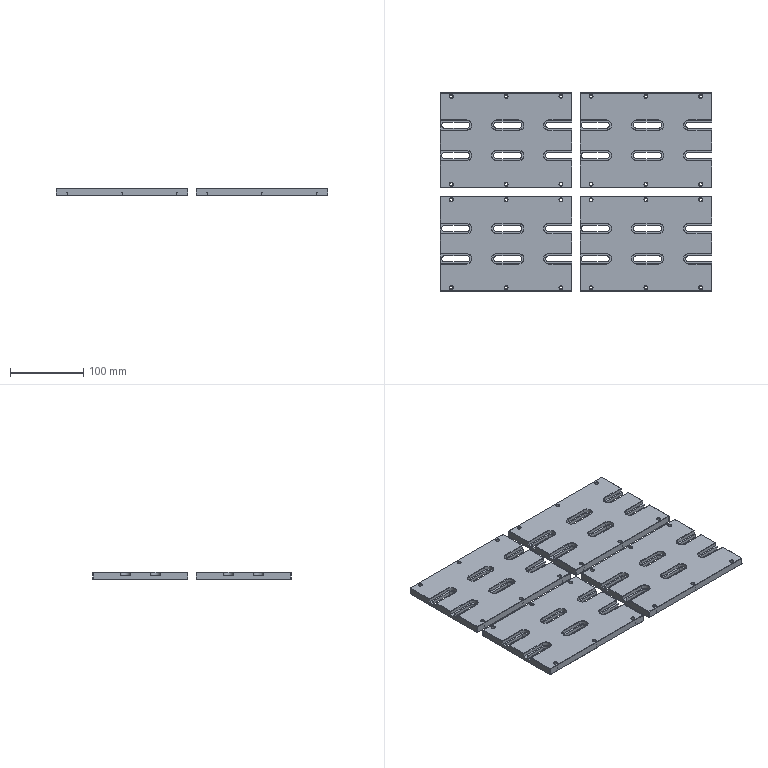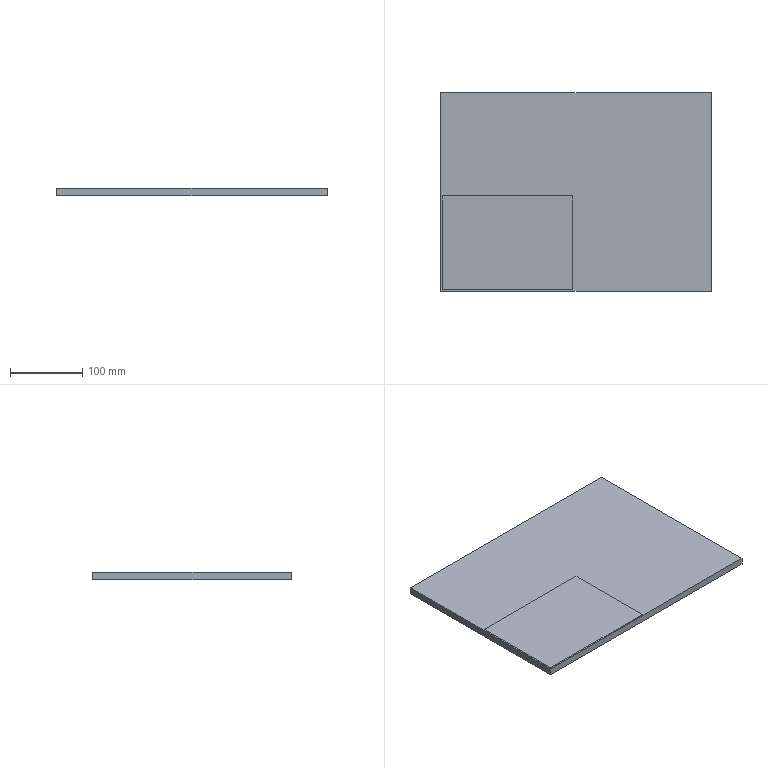CAM job | NX | 3-axis milling, drilling | part box 371 x 271 x 10 mm | stock box 375 x 275 x 10 mm
Tools:
number,name,description,diameter,corner_radius,flute_length,length,flutes
2,D4A45,Milling Tool-5 Parameters,4.0,0.0,2.0,2.0,2
14,4.5ZT,Drilling Tool,4.0,0.0,35.0,50.0,2
10,D10JING,Milling Tool-5 Parameters,10.0,0.0,50.0,75.0,2
6,D6,Milling Tool-5 Parameters,6.0,0.0,50.0,75.0,2
Operations:
program,operation,operation_type,tool,method,geometry_group,spindle_rpm,surface_speed,feed_per_tooth,feed_cut,feed_plunge,cut_length_mm,path_length_mm,cut_time_min,machine_time_min
1吸,DRILLING_COPY,Operation,D4A45,METHOD,A,5000.0,62.0,0.025,250.0,0.0,96.0,1715.285,0.384,0.5459
1吸,DRILLING_COPY_COPY_COPY_COPY,Operation,4.5ZT,METHOD,A,1910.0,21.0,0.0471,180.0,0.0,258.041,2039.368,1.434,1.612
1吸,ZLEVEL_PROFILE_1_COPY_1_COPY,ZLevelMilling,D4A45,METHOD,A,9500.0,179.0,0.0526,1000.0,100.0,4910.138,11150.585,4.91,5.534
1吸,ZLEVEL_PROFILE,ZLevelMilling,D6,METHOD,A,9500.0,179.0,0.1579,3000.0,1000.0,52971.052,54041.533,17.762,17.87
1吸,ZLEVEL_PROFILE_1,ZLevelMilling,D10JING,METHOD,A,9500.0,298.0,0.0789,1500.0,1000.0,3658.225,4802.999,2.566,2.681
1吸,ZLEVEL_PROFILE_1_COPY,ZLevelMilling,D10JING,METHOD,A,9500.0,298.0,0.0789,1500.0,1000.0,6968.348,9113.93,4.692,4.907
1吸,ZLEVEL_PROFILE_COPY_COPY,ZLevelMilling,D6,METHOD,A,9500.0,119.0,0.0632,1200.0,1000.0,3120.922,4502.514,2.603,2.741
2,ZLEVEL_PROFILE_1_COPY_1_COPY_COPY,ZLevelMilling,D4A45,METHOD,B,9500.0,179.0,0.0526,1000.0,100.0,1277.493,2894.152,1.278,1.439
2,ZLEVEL_PROFILE_1_COPY_1,ZLevelMilling,D6,METHOD,B,9500.0,298.0,0.0789,1500.0,1000.0,2731.226,3128.593,1.873,1.913
2,HOLE_MILLING,CylinderMilling,D6,METHOD,B,9500.0,179.0,0.0658,1250.0,100.0,492.08,1388.78,0.3937,0.4833